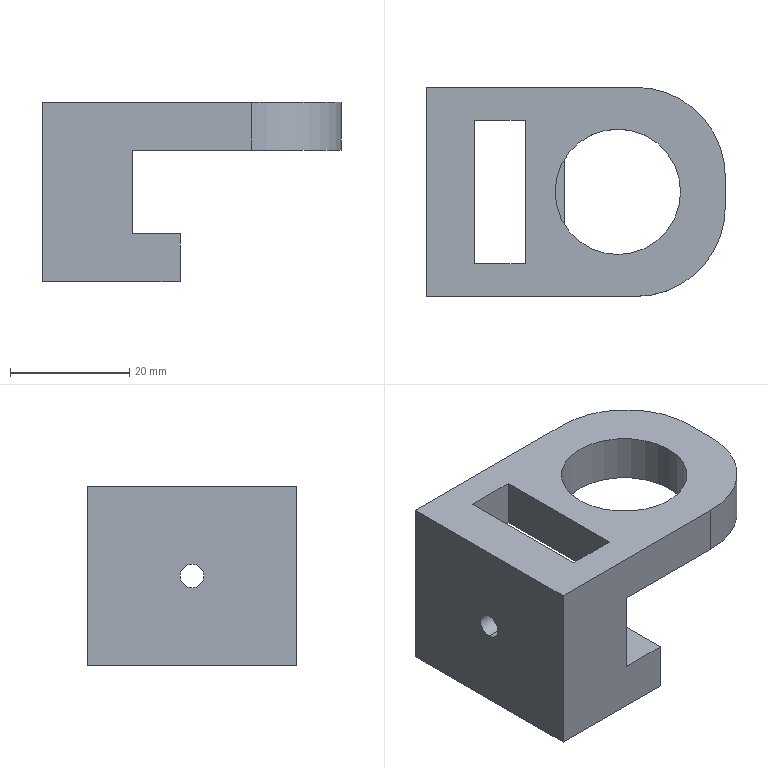Part | STEP file | X77-04004 | 1 solid | 22 faces | box 50 x 35 x 30 mm | volume 18530 mm3 | plane 16 | cylinder 6 | commonest cylinder face diameters 4 x2 21 x2 30 x2
STEP:
#1=CARTESIAN_POINT('',(0.,17.5,17.));
#2=VERTEX_POINT('',#1);
#3=CARTESIAN_POINT('',(0.,17.5,13.));
#4=VERTEX_POINT('',#3);
#5=CARTESIAN_POINT('',(0.,17.5,15.));
#6=DIRECTION('',(1.,0.,0.));
#7=DIRECTION('',(0.,0.,-1.));
#8=AXIS2_PLACEMENT_3D('',#5,#6,#7);
#9=CIRCLE('',#8,2.);
#10=EDGE_CURVE('',#2,#4,#9,.T.);
#11=ORIENTED_EDGE('',*,*,#10,.F.);
#12=CARTESIAN_POINT('',(8.,17.5,17.));
#13=VERTEX_POINT('',#12);
#14=CARTESIAN_POINT('',(8.,17.5,17.));
#15=DIRECTION('',(1.,0.,0.));
#16=VECTOR('',#15,1000.);
#17=LINE('',#14,#16);
#18=EDGE_CURVE('',#2,#13,#17,.T.);
#19=ORIENTED_EDGE('',*,*,#18,.T.);
#20=CARTESIAN_POINT('',(8.,17.5,13.));
#21=VERTEX_POINT('',#20);
#22=CARTESIAN_POINT('',(8.,17.5,15.));
#23=DIRECTION('',(1.,0.,0.));
#24=DIRECTION('',(0.,0.,-1.));
#25=AXIS2_PLACEMENT_3D('',#22,#23,#24);
#26=CIRCLE('',#25,2.);
#27=EDGE_CURVE('',#13,#21,#26,.T.);
#28=ORIENTED_EDGE('',*,*,#27,.T.);
#29=CARTESIAN_POINT('',(8.,17.5,13.));
#30=DIRECTION('',(1.,0.,0.));
#31=VECTOR('',#30,1000.);
#32=LINE('',#29,#31);
#33=EDGE_CURVE('',#4,#21,#32,.T.);
#34=ORIENTED_EDGE('',*,*,#33,.F.);
#35=EDGE_LOOP('',(#11,#19,#28,#34));
#36=FACE_OUTER_BOUND('',#35,.T.);
#37=CARTESIAN_POINT('',(8.,17.5,15.));
#38=DIRECTION('',(1.,0.,0.));
#39=DIRECTION('',(0.,0.,-1.));
#40=AXIS2_PLACEMENT_3D('',#37,#38,#39);
#41=CYLINDRICAL_SURFACE('',#40,2.);
#42=ADVANCED_FACE('',(#36),#41,.F.);
#43=CARTESIAN_POINT('',(42.5,17.5,22.));
#44=VERTEX_POINT('',#43);
#45=CARTESIAN_POINT('',(21.5,17.5,22.));
#46=VERTEX_POINT('',#45);
#47=CARTESIAN_POINT('',(32.,17.5,22.));
#48=DIRECTION('',(0.,0.,-1.));
#49=DIRECTION('',(1.,0.,0.));
#50=AXIS2_PLACEMENT_3D('',#47,#48,#49);
#51=CIRCLE('',#50,10.5);
#52=EDGE_CURVE('',#44,#46,#51,.T.);
#53=ORIENTED_EDGE('',*,*,#52,.T.);
#54=CARTESIAN_POINT('',(21.5,17.5,30.));
#55=VERTEX_POINT('',#54);
#56=CARTESIAN_POINT('',(21.5,17.5,-0.001));
#57=DIRECTION('',(0.,0.,1.));
#58=VECTOR('',#57,1000.);
#59=LINE('',#56,#58);
#60=EDGE_CURVE('',#46,#55,#59,.T.);
#61=ORIENTED_EDGE('',*,*,#60,.T.);
#62=CARTESIAN_POINT('',(42.5,17.5,30.));
#63=VERTEX_POINT('',#62);
#64=CARTESIAN_POINT('',(32.,17.5,30.));
#65=DIRECTION('',(0.,0.,1.));
#66=DIRECTION('',(1.,0.,0.));
#67=AXIS2_PLACEMENT_3D('',#64,#65,#66);
#68=CIRCLE('',#67,10.5);
#69=EDGE_CURVE('',#55,#63,#68,.T.);
#70=ORIENTED_EDGE('',*,*,#69,.T.);
#71=CARTESIAN_POINT('',(42.5,17.5,-0.001));
#72=DIRECTION('',(0.,0.,1.));
#73=VECTOR('',#72,1000.);
#74=LINE('',#71,#73);
#75=EDGE_CURVE('',#44,#63,#74,.T.);
#76=ORIENTED_EDGE('',*,*,#75,.F.);
#77=EDGE_LOOP('',(#53,#61,#70,#76));
#78=FACE_OUTER_BOUND('',#77,.T.);
#79=CARTESIAN_POINT('',(32.,17.5,-0.001));
#80=DIRECTION('',(0.,0.,1.));
#81=DIRECTION('',(1.,0.,0.));
#82=AXIS2_PLACEMENT_3D('',#79,#80,#81);
#83=CYLINDRICAL_SURFACE('',#82,10.5);
#84=ADVANCED_FACE('',(#78),#83,.F.);
#85=CARTESIAN_POINT('',(16.5,5.5,22.));
#86=VERTEX_POINT('',#85);
#87=CARTESIAN_POINT('',(16.5,29.5,22.));
#88=VERTEX_POINT('',#87);
#89=CARTESIAN_POINT('',(16.5,29.5,22.));
#90=DIRECTION('',(0.,1.,0.));
#91=VECTOR('',#90,1000.);
#92=LINE('',#89,#91);
#93=EDGE_CURVE('',#86,#88,#92,.T.);
#94=ORIENTED_EDGE('',*,*,#93,.F.);
#95=CARTESIAN_POINT('',(16.5,5.5,30.));
#96=VERTEX_POINT('',#95);
#97=CARTESIAN_POINT('',(16.5,5.5,30.));
#98=DIRECTION('',(0.,0.,-1.));
#99=VECTOR('',#98,1000.);
#100=LINE('',#97,#99);
#101=EDGE_CURVE('',#96,#86,#100,.T.);
#102=ORIENTED_EDGE('',*,*,#101,.F.);
#103=CARTESIAN_POINT('',(16.5,29.5,30.));
#104=VERTEX_POINT('',#103);
#105=CARTESIAN_POINT('',(16.5,29.5,30.));
#106=DIRECTION('',(0.,1.,0.));
#107=VECTOR('',#106,1000.);
#108=LINE('',#105,#107);
#109=EDGE_CURVE('',#96,#104,#108,.T.);
#110=ORIENTED_EDGE('',*,*,#109,.T.);
#111=CARTESIAN_POINT('',(16.5,29.5,30.));
#112=DIRECTION('',(0.,0.,-1.));
#113=VECTOR('',#112,1000.);
#114=LINE('',#111,#113);
#115=EDGE_CURVE('',#104,#88,#114,.T.);
#116=ORIENTED_EDGE('',*,*,#115,.T.);
#117=EDGE_LOOP('',(#94,#102,#110,#116));
#118=FACE_OUTER_BOUND('',#117,.T.);
#119=CARTESIAN_POINT('',(16.5,29.5,30.));
#120=DIRECTION('',(-1.,0.,0.));
#121=DIRECTION('',(0.,-1.,0.));
#122=AXIS2_PLACEMENT_3D('',#119,#120,#121);
#123=PLANE('',#122);
#124=ADVANCED_FACE('',(#118),#123,.T.);
#125=CARTESIAN_POINT('',(32.,17.5,30.));
#126=DIRECTION('',(0.,0.,1.));
#127=DIRECTION('',(1.,0.,0.));
#128=AXIS2_PLACEMENT_3D('',#125,#126,#127);
#129=CIRCLE('',#128,10.5);
#130=EDGE_CURVE('',#63,#55,#129,.T.);
#131=ORIENTED_EDGE('',*,*,#130,.F.);
#132=ORIENTED_EDGE('',*,*,#69,.F.);
#133=EDGE_LOOP('',(#131,#132));
#134=FACE_BOUND('',#133,.T.);
#135=CARTESIAN_POINT('',(0.,0.,30.));
#136=VERTEX_POINT('',#135);
#137=CARTESIAN_POINT('',(35.,0.,30.));
#138=VERTEX_POINT('',#137);
#139=CARTESIAN_POINT('',(0.,0.,30.));
#140=DIRECTION('',(1.,0.,0.));
#141=VECTOR('',#140,1000.);
#142=LINE('',#139,#141);
#143=EDGE_CURVE('',#136,#138,#142,.T.);
#144=ORIENTED_EDGE('',*,*,#143,.T.);
#145=CARTESIAN_POINT('',(50.,15.,30.));
#146=VERTEX_POINT('',#145);
#147=CARTESIAN_POINT('',(35.,15.,30.));
#148=DIRECTION('',(0.,0.,1.));
#149=DIRECTION('',(-1.,0.,0.));
#150=AXIS2_PLACEMENT_3D('',#147,#148,#149);
#151=CIRCLE('',#150,15.);
#152=EDGE_CURVE('',#138,#146,#151,.T.);
#153=ORIENTED_EDGE('',*,*,#152,.T.);
#154=CARTESIAN_POINT('',(50.,20.,30.));
#155=VERTEX_POINT('',#154);
#156=CARTESIAN_POINT('',(50.,0.,30.));
#157=DIRECTION('',(0.,1.,0.));
#158=VECTOR('',#157,1000.);
#159=LINE('',#156,#158);
#160=EDGE_CURVE('',#146,#155,#159,.T.);
#161=ORIENTED_EDGE('',*,*,#160,.T.);
#162=CARTESIAN_POINT('',(35.,35.,30.));
#163=VERTEX_POINT('',#162);
#164=CARTESIAN_POINT('',(35.,20.,30.));
#165=DIRECTION('',(0.,0.,1.));
#166=DIRECTION('',(-1.,0.,0.));
#167=AXIS2_PLACEMENT_3D('',#164,#165,#166);
#168=CIRCLE('',#167,15.);
#169=EDGE_CURVE('',#155,#163,#168,.T.);
#170=ORIENTED_EDGE('',*,*,#169,.T.);
#171=CARTESIAN_POINT('',(0.,35.,30.));
#172=VERTEX_POINT('',#171);
#173=CARTESIAN_POINT('',(0.,35.,30.));
#174=DIRECTION('',(-1.,0.,0.));
#175=VECTOR('',#174,1000.);
#176=LINE('',#173,#175);
#177=EDGE_CURVE('',#163,#172,#176,.T.);
#178=ORIENTED_EDGE('',*,*,#177,.T.);
#179=CARTESIAN_POINT('',(0.,0.,30.));
#180=DIRECTION('',(0.,-1.,0.));
#181=VECTOR('',#180,1000.);
#182=LINE('',#179,#181);
#183=EDGE_CURVE('',#172,#136,#182,.T.);
#184=ORIENTED_EDGE('',*,*,#183,.T.);
#185=EDGE_LOOP('',(#144,#153,#161,#170,#178,#184));
#186=FACE_OUTER_BOUND('',#185,.T.);
#187=CARTESIAN_POINT('',(8.,29.5,30.));
#188=VERTEX_POINT('',#187);
#189=CARTESIAN_POINT('',(8.,5.5,30.));
#190=VERTEX_POINT('',#189);
#191=CARTESIAN_POINT('',(8.,29.5,30.));
#192=DIRECTION('',(0.,-1.,0.));
#193=VECTOR('',#192,1000.);
#194=LINE('',#191,#193);
#195=EDGE_CURVE('',#188,#190,#194,.T.);
#196=ORIENTED_EDGE('',*,*,#195,.F.);
#197=CARTESIAN_POINT('',(8.,29.5,30.));
#198=DIRECTION('',(-1.,0.,0.));
#199=VECTOR('',#198,1000.);
#200=LINE('',#197,#199);
#201=EDGE_CURVE('',#104,#188,#200,.T.);
#202=ORIENTED_EDGE('',*,*,#201,.F.);
#203=ORIENTED_EDGE('',*,*,#109,.F.);
#204=CARTESIAN_POINT('',(8.,5.5,30.));
#205=DIRECTION('',(1.,0.,0.));
#206=VECTOR('',#205,1000.);
#207=LINE('',#204,#206);
#208=EDGE_CURVE('',#190,#96,#207,.T.);
#209=ORIENTED_EDGE('',*,*,#208,.F.);
#210=EDGE_LOOP('',(#196,#202,#203,#209));
#211=FACE_BOUND('',#210,.T.);
#212=CARTESIAN_POINT('',(0.,35.,30.));
#213=DIRECTION('',(0.,0.,-1.));
#214=DIRECTION('',(-1.,0.,0.));
#215=AXIS2_PLACEMENT_3D('',#212,#213,#214);
#216=PLANE('',#215);
#217=ADVANCED_FACE('',(#134,#186,#211),#216,.F.);
#218=CARTESIAN_POINT('',(23.,35.,0.));
#219=VERTEX_POINT('',#218);
#220=CARTESIAN_POINT('',(23.,0.,0.));
#221=VERTEX_POINT('',#220);
#222=CARTESIAN_POINT('',(23.,44.,0.));
#223=DIRECTION('',(0.,-1.,0.));
#224=VECTOR('',#223,1000.);
#225=LINE('',#222,#224);
#226=EDGE_CURVE('',#219,#221,#225,.T.);
#227=ORIENTED_EDGE('',*,*,#226,.T.);
#228=CARTESIAN_POINT('',(0.,0.,0.));
#229=VERTEX_POINT('',#228);
#230=CARTESIAN_POINT('',(0.,0.,0.));
#231=DIRECTION('',(1.,0.,0.));
#232=VECTOR('',#231,1000.);
#233=LINE('',#230,#232);
#234=EDGE_CURVE('',#229,#221,#233,.T.);
#235=ORIENTED_EDGE('',*,*,#234,.F.);
#236=CARTESIAN_POINT('',(0.,35.,0.));
#237=VERTEX_POINT('',#236);
#238=CARTESIAN_POINT('',(0.,0.,0.));
#239=DIRECTION('',(0.,-1.,0.));
#240=VECTOR('',#239,1000.);
#241=LINE('',#238,#240);
#242=EDGE_CURVE('',#237,#229,#241,.T.);
#243=ORIENTED_EDGE('',*,*,#242,.F.);
#244=CARTESIAN_POINT('',(0.,35.,0.));
#245=DIRECTION('',(-1.,0.,0.));
#246=VECTOR('',#245,1000.);
#247=LINE('',#244,#246);
#248=EDGE_CURVE('',#219,#237,#247,.T.);
#249=ORIENTED_EDGE('',*,*,#248,.F.);
#250=EDGE_LOOP('',(#227,#235,#243,#249));
#251=FACE_OUTER_BOUND('',#250,.T.);
#252=CARTESIAN_POINT('',(16.5,29.5,0.));
#253=VERTEX_POINT('',#252);
#254=CARTESIAN_POINT('',(8.,29.5,0.));
#255=VERTEX_POINT('',#254);
#256=CARTESIAN_POINT('',(8.,29.5,0.));
#257=DIRECTION('',(-1.,0.,0.));
#258=VECTOR('',#257,1000.);
#259=LINE('',#256,#258);
#260=EDGE_CURVE('',#253,#255,#259,.T.);
#261=ORIENTED_EDGE('',*,*,#260,.T.);
#262=CARTESIAN_POINT('',(8.,5.5,0.));
#263=VERTEX_POINT('',#262);
#264=CARTESIAN_POINT('',(8.,29.5,0.));
#265=DIRECTION('',(0.,-1.,0.));
#266=VECTOR('',#265,1000.);
#267=LINE('',#264,#266);
#268=EDGE_CURVE('',#255,#263,#267,.T.);
#269=ORIENTED_EDGE('',*,*,#268,.T.);
#270=CARTESIAN_POINT('',(16.5,5.5,0.));
#271=VERTEX_POINT('',#270);
#272=CARTESIAN_POINT('',(8.,5.5,0.));
#273=DIRECTION('',(1.,0.,0.));
#274=VECTOR('',#273,1000.);
#275=LINE('',#272,#274);
#276=EDGE_CURVE('',#263,#271,#275,.T.);
#277=ORIENTED_EDGE('',*,*,#276,.T.);
#278=CARTESIAN_POINT('',(16.5,29.5,0.));
#279=DIRECTION('',(0.,1.,0.));
#280=VECTOR('',#279,1000.);
#281=LINE('',#278,#280);
#282=EDGE_CURVE('',#271,#253,#281,.T.);
#283=ORIENTED_EDGE('',*,*,#282,.T.);
#284=EDGE_LOOP('',(#261,#269,#277,#283));
#285=FACE_BOUND('',#284,.T.);
#286=CARTESIAN_POINT('',(0.,35.,0.));
#287=DIRECTION('',(0.,0.,-1.));
#288=DIRECTION('',(-1.,0.,0.));
#289=AXIS2_PLACEMENT_3D('',#286,#287,#288);
#290=PLANE('',#289);
#291=ADVANCED_FACE('',(#251,#285),#290,.T.);
#292=CARTESIAN_POINT('',(0.,17.5,15.));
#293=DIRECTION('',(1.,0.,0.));
#294=DIRECTION('',(0.,0.,-1.));
#295=AXIS2_PLACEMENT_3D('',#292,#293,#294);
#296=CIRCLE('',#295,2.);
#297=EDGE_CURVE('',#4,#2,#296,.T.);
#298=ORIENTED_EDGE('',*,*,#297,.T.);
#299=ORIENTED_EDGE('',*,*,#10,.T.);
#300=EDGE_LOOP('',(#298,#299));
#301=FACE_BOUND('',#300,.T.);
#302=ORIENTED_EDGE('',*,*,#242,.T.);
#303=CARTESIAN_POINT('',(0.,0.,30.));
#304=DIRECTION('',(0.,0.,-1.));
#305=VECTOR('',#304,1000.);
#306=LINE('',#303,#305);
#307=EDGE_CURVE('',#136,#229,#306,.T.);
#308=ORIENTED_EDGE('',*,*,#307,.F.);
#309=ORIENTED_EDGE('',*,*,#183,.F.);
#310=CARTESIAN_POINT('',(0.,35.,30.));
#311=DIRECTION('',(0.,0.,-1.));
#312=VECTOR('',#311,1000.);
#313=LINE('',#310,#312);
#314=EDGE_CURVE('',#172,#237,#313,.T.);
#315=ORIENTED_EDGE('',*,*,#314,.T.);
#316=EDGE_LOOP('',(#302,#308,#309,#315));
#317=FACE_OUTER_BOUND('',#316,.T.);
#318=CARTESIAN_POINT('',(0.,0.,30.));
#319=DIRECTION('',(1.,0.,0.));
#320=DIRECTION('',(0.,0.,-1.));
#321=AXIS2_PLACEMENT_3D('',#318,#319,#320);
#322=PLANE('',#321);
#323=ADVANCED_FACE('',(#301,#317),#322,.F.);
#324=CARTESIAN_POINT('',(35.,0.,22.));
#325=VERTEX_POINT('',#324);
#326=CARTESIAN_POINT('',(15.,0.,22.));
#327=VERTEX_POINT('',#326);
#328=CARTESIAN_POINT('',(50.,0.,22.));
#329=DIRECTION('',(-1.,0.,0.));
#330=VECTOR('',#329,1000.);
#331=LINE('',#328,#330);
#332=EDGE_CURVE('',#325,#327,#331,.T.);
#333=ORIENTED_EDGE('',*,*,#332,.F.);
#334=CARTESIAN_POINT('',(35.,0.,30.));
#335=DIRECTION('',(0.,0.,1.));
#336=VECTOR('',#335,1000.);
#337=LINE('',#334,#336);
#338=EDGE_CURVE('',#325,#138,#337,.T.);
#339=ORIENTED_EDGE('',*,*,#338,.T.);
#340=ORIENTED_EDGE('',*,*,#143,.F.);
#341=ORIENTED_EDGE('',*,*,#307,.T.);
#342=ORIENTED_EDGE('',*,*,#234,.T.);
#343=CARTESIAN_POINT('',(23.,0.,8.));
#344=VERTEX_POINT('',#343);
#345=CARTESIAN_POINT('',(23.,0.,8.));
#346=DIRECTION('',(0.,0.,-1.));
#347=VECTOR('',#346,1000.);
#348=LINE('',#345,#347);
#349=EDGE_CURVE('',#344,#221,#348,.T.);
#350=ORIENTED_EDGE('',*,*,#349,.F.);
#351=CARTESIAN_POINT('',(15.,0.,8.));
#352=VERTEX_POINT('',#351);
#353=CARTESIAN_POINT('',(23.,0.,8.));
#354=DIRECTION('',(1.,0.,0.));
#355=VECTOR('',#354,1000.);
#356=LINE('',#353,#355);
#357=EDGE_CURVE('',#352,#344,#356,.T.);
#358=ORIENTED_EDGE('',*,*,#357,.F.);
#359=CARTESIAN_POINT('',(15.,0.,8.));
#360=DIRECTION('',(0.,0.,-1.));
#361=VECTOR('',#360,1000.);
#362=LINE('',#359,#361);
#363=EDGE_CURVE('',#327,#352,#362,.T.);
#364=ORIENTED_EDGE('',*,*,#363,.F.);
#365=EDGE_LOOP('',(#333,#339,#340,#341,#342,#350,#358,#364));
#366=FACE_OUTER_BOUND('',#365,.T.);
#367=CARTESIAN_POINT('',(0.,0.,30.));
#368=DIRECTION('',(0.,1.,0.));
#369=DIRECTION('',(0.,0.,1.));
#370=AXIS2_PLACEMENT_3D('',#367,#368,#369);
#371=PLANE('',#370);
#372=ADVANCED_FACE('',(#366),#371,.F.);
#373=ORIENTED_EDGE('',*,*,#160,.F.);
#374=CARTESIAN_POINT('',(50.,15.,22.));
#375=VERTEX_POINT('',#374);
#376=CARTESIAN_POINT('',(50.,15.,30.));
#377=DIRECTION('',(0.,0.,-1.));
#378=VECTOR('',#377,1000.);
#379=LINE('',#376,#378);
#380=EDGE_CURVE('',#146,#375,#379,.T.);
#381=ORIENTED_EDGE('',*,*,#380,.T.);
#382=CARTESIAN_POINT('',(50.,20.,22.));
#383=VERTEX_POINT('',#382);
#384=CARTESIAN_POINT('',(50.,44.,22.));
#385=DIRECTION('',(0.,-1.,0.));
#386=VECTOR('',#385,1000.);
#387=LINE('',#384,#386);
#388=EDGE_CURVE('',#383,#375,#387,.T.);
#389=ORIENTED_EDGE('',*,*,#388,.F.);
#390=CARTESIAN_POINT('',(50.,20.,30.));
#391=DIRECTION('',(0.,0.,1.));
#392=VECTOR('',#391,1000.);
#393=LINE('',#390,#392);
#394=EDGE_CURVE('',#383,#155,#393,.T.);
#395=ORIENTED_EDGE('',*,*,#394,.T.);
#396=EDGE_LOOP('',(#373,#381,#389,#395));
#397=FACE_OUTER_BOUND('',#396,.T.);
#398=CARTESIAN_POINT('',(50.,0.,30.));
#399=DIRECTION('',(-1.,0.,0.));
#400=DIRECTION('',(0.,0.,1.));
#401=AXIS2_PLACEMENT_3D('',#398,#399,#400);
#402=PLANE('',#401);
#403=ADVANCED_FACE('',(#397),#402,.F.);
#404=ORIENTED_EDGE('',*,*,#177,.F.);
#405=CARTESIAN_POINT('',(35.,35.,22.));
#406=VERTEX_POINT('',#405);
#407=CARTESIAN_POINT('',(35.,35.,30.));
#408=DIRECTION('',(0.,0.,-1.));
#409=VECTOR('',#408,1000.);
#410=LINE('',#407,#409);
#411=EDGE_CURVE('',#163,#406,#410,.T.);
#412=ORIENTED_EDGE('',*,*,#411,.T.);
#413=CARTESIAN_POINT('',(15.,35.,22.));
#414=VERTEX_POINT('',#413);
#415=CARTESIAN_POINT('',(0.,35.,22.));
#416=DIRECTION('',(-1.,0.,0.));
#417=VECTOR('',#416,1000.);
#418=LINE('',#415,#417);
#419=EDGE_CURVE('',#406,#414,#418,.T.);
#420=ORIENTED_EDGE('',*,*,#419,.T.);
#421=CARTESIAN_POINT('',(15.,35.,8.));
#422=VERTEX_POINT('',#421);
#423=CARTESIAN_POINT('',(15.,35.,30.));
#424=DIRECTION('',(0.,0.,-1.));
#425=VECTOR('',#424,1000.);
#426=LINE('',#423,#425);
#427=EDGE_CURVE('',#414,#422,#426,.T.);
#428=ORIENTED_EDGE('',*,*,#427,.T.);
#429=CARTESIAN_POINT('',(23.,35.,8.));
#430=VERTEX_POINT('',#429);
#431=CARTESIAN_POINT('',(0.,35.,8.));
#432=DIRECTION('',(1.,0.,0.));
#433=VECTOR('',#432,1000.);
#434=LINE('',#431,#433);
#435=EDGE_CURVE('',#422,#430,#434,.T.);
#436=ORIENTED_EDGE('',*,*,#435,.T.);
#437=CARTESIAN_POINT('',(23.,35.,30.));
#438=DIRECTION('',(0.,0.,-1.));
#439=VECTOR('',#438,1000.);
#440=LINE('',#437,#439);
#441=EDGE_CURVE('',#430,#219,#440,.T.);
#442=ORIENTED_EDGE('',*,*,#441,.T.);
#443=ORIENTED_EDGE('',*,*,#248,.T.);
#444=ORIENTED_EDGE('',*,*,#314,.F.);
#445=EDGE_LOOP('',(#404,#412,#420,#428,#436,#442,#443,#444));
#446=FACE_OUTER_BOUND('',#445,.T.);
#447=CARTESIAN_POINT('',(0.,35.,30.));
#448=DIRECTION('',(0.,-1.,0.));
#449=DIRECTION('',(0.,0.,-1.));
#450=AXIS2_PLACEMENT_3D('',#447,#448,#449);
#451=PLANE('',#450);
#452=ADVANCED_FACE('',(#446),#451,.F.);
#453=CARTESIAN_POINT('',(8.,17.5,15.));
#454=DIRECTION('',(1.,0.,0.));
#455=DIRECTION('',(0.,0.,-1.));
#456=AXIS2_PLACEMENT_3D('',#453,#454,#455);
#457=CIRCLE('',#456,2.);
#458=EDGE_CURVE('',#21,#13,#457,.T.);
#459=ORIENTED_EDGE('',*,*,#458,.F.);
#460=ORIENTED_EDGE('',*,*,#27,.F.);
#461=EDGE_LOOP('',(#459,#460));
#462=FACE_BOUND('',#461,.T.);
#463=ORIENTED_EDGE('',*,*,#268,.F.);
#464=CARTESIAN_POINT('',(8.,29.5,30.));
#465=DIRECTION('',(0.,0.,-1.));
#466=VECTOR('',#465,1000.);
#467=LINE('',#464,#466);
#468=EDGE_CURVE('',#188,#255,#467,.T.);
#469=ORIENTED_EDGE('',*,*,#468,.F.);
#470=ORIENTED_EDGE('',*,*,#195,.T.);
#471=CARTESIAN_POINT('',(8.,5.5,30.));
#472=DIRECTION('',(0.,0.,-1.));
#473=VECTOR('',#472,1000.);
#474=LINE('',#471,#473);
#475=EDGE_CURVE('',#190,#263,#474,.T.);
#476=ORIENTED_EDGE('',*,*,#475,.T.);
#477=EDGE_LOOP('',(#463,#469,#470,#476));
#478=FACE_OUTER_BOUND('',#477,.T.);
#479=CARTESIAN_POINT('',(8.,29.5,30.));
#480=DIRECTION('',(1.,0.,0.));
#481=DIRECTION('',(0.,1.,0.));
#482=AXIS2_PLACEMENT_3D('',#479,#480,#481);
#483=PLANE('',#482);
#484=ADVANCED_FACE('',(#462,#478),#483,.T.);
#485=CARTESIAN_POINT('',(15.,5.5,22.));
#486=VERTEX_POINT('',#485);
#487=CARTESIAN_POINT('',(8.,5.5,22.));
#488=DIRECTION('',(1.,0.,0.));
#489=VECTOR('',#488,1000.);
#490=LINE('',#487,#489);
#491=EDGE_CURVE('',#486,#86,#490,.T.);
#492=ORIENTED_EDGE('',*,*,#491,.F.);
#493=CARTESIAN_POINT('',(15.,5.5,8.));
#494=VERTEX_POINT('',#493);
#495=CARTESIAN_POINT('',(15.,5.5,30.));
#496=DIRECTION('',(0.,0.,1.));
#497=VECTOR('',#496,1000.);
#498=LINE('',#495,#497);
#499=EDGE_CURVE('',#494,#486,#498,.T.);
#500=ORIENTED_EDGE('',*,*,#499,.F.);
#501=CARTESIAN_POINT('',(16.5,5.5,8.));
#502=VERTEX_POINT('',#501);
#503=CARTESIAN_POINT('',(8.,5.5,8.));
#504=DIRECTION('',(-1.,0.,0.));
#505=VECTOR('',#504,1000.);
#506=LINE('',#503,#505);
#507=EDGE_CURVE('',#502,#494,#506,.T.);
#508=ORIENTED_EDGE('',*,*,#507,.F.);
#509=CARTESIAN_POINT('',(16.5,5.5,30.));
#510=DIRECTION('',(0.,0.,-1.));
#511=VECTOR('',#510,1000.);
#512=LINE('',#509,#511);
#513=EDGE_CURVE('',#502,#271,#512,.T.);
#514=ORIENTED_EDGE('',*,*,#513,.T.);
#515=ORIENTED_EDGE('',*,*,#276,.F.);
#516=ORIENTED_EDGE('',*,*,#475,.F.);
#517=ORIENTED_EDGE('',*,*,#208,.T.);
#518=ORIENTED_EDGE('',*,*,#101,.T.);
#519=EDGE_LOOP('',(#492,#500,#508,#514,#515,#516,#517,#518));
#520=FACE_OUTER_BOUND('',#519,.T.);
#521=CARTESIAN_POINT('',(8.,5.5,30.));
#522=DIRECTION('',(0.,1.,0.));
#523=DIRECTION('',(0.,0.,1.));
#524=AXIS2_PLACEMENT_3D('',#521,#522,#523);
#525=PLANE('',#524);
#526=ADVANCED_FACE('',(#520),#525,.T.);
#527=CARTESIAN_POINT('',(16.5,29.5,8.));
#528=VERTEX_POINT('',#527);
#529=CARTESIAN_POINT('',(16.5,29.5,8.));
#530=DIRECTION('',(0.,-1.,0.));
#531=VECTOR('',#530,1000.);
#532=LINE('',#529,#531);
#533=EDGE_CURVE('',#528,#502,#532,.T.);
#534=ORIENTED_EDGE('',*,*,#533,.F.);
#535=CARTESIAN_POINT('',(16.5,29.5,30.));
#536=DIRECTION('',(0.,0.,-1.));
#537=VECTOR('',#536,1000.);
#538=LINE('',#535,#537);
#539=EDGE_CURVE('',#528,#253,#538,.T.);
#540=ORIENTED_EDGE('',*,*,#539,.T.);
#541=ORIENTED_EDGE('',*,*,#282,.F.);
#542=ORIENTED_EDGE('',*,*,#513,.F.);
#543=EDGE_LOOP('',(#534,#540,#541,#542));
#544=FACE_OUTER_BOUND('',#543,.T.);
#545=CARTESIAN_POINT('',(16.5,29.5,30.));
#546=DIRECTION('',(-1.,0.,0.));
#547=DIRECTION('',(0.,-1.,0.));
#548=AXIS2_PLACEMENT_3D('',#545,#546,#547);
#549=PLANE('',#548);
#550=ADVANCED_FACE('',(#544),#549,.T.);
#551=CARTESIAN_POINT('',(15.,29.5,22.));
#552=VERTEX_POINT('',#551);
#553=CARTESIAN_POINT('',(8.,29.5,22.));
#554=DIRECTION('',(-1.,0.,0.));
#555=VECTOR('',#554,1000.);
#556=LINE('',#553,#555);
#557=EDGE_CURVE('',#88,#552,#556,.T.);
#558=ORIENTED_EDGE('',*,*,#557,.F.);
#559=ORIENTED_EDGE('',*,*,#115,.F.);
#560=ORIENTED_EDGE('',*,*,#201,.T.);
#561=ORIENTED_EDGE('',*,*,#468,.T.);
#562=ORIENTED_EDGE('',*,*,#260,.F.);
#563=ORIENTED_EDGE('',*,*,#539,.F.);
#564=CARTESIAN_POINT('',(15.,29.5,8.));
#565=VERTEX_POINT('',#564);
#566=CARTESIAN_POINT('',(8.,29.5,8.));
#567=DIRECTION('',(1.,0.,0.));
#568=VECTOR('',#567,1000.);
#569=LINE('',#566,#568);
#570=EDGE_CURVE('',#565,#528,#569,.T.);
#571=ORIENTED_EDGE('',*,*,#570,.F.);
#572=CARTESIAN_POINT('',(15.,29.5,30.));
#573=DIRECTION('',(0.,0.,-1.));
#574=VECTOR('',#573,1000.);
#575=LINE('',#572,#574);
#576=EDGE_CURVE('',#552,#565,#575,.T.);
#577=ORIENTED_EDGE('',*,*,#576,.F.);
#578=EDGE_LOOP('',(#558,#559,#560,#561,#562,#563,#571,#577));
#579=FACE_OUTER_BOUND('',#578,.T.);
#580=CARTESIAN_POINT('',(8.,29.5,30.));
#581=DIRECTION('',(0.,-1.,0.));
#582=DIRECTION('',(0.,0.,-1.));
#583=AXIS2_PLACEMENT_3D('',#580,#581,#582);
#584=PLANE('',#583);
#585=ADVANCED_FACE('',(#579),#584,.T.);
#586=CARTESIAN_POINT('',(23.,44.,8.));
#587=DIRECTION('',(0.,-1.,0.));
#588=VECTOR('',#587,1000.);
#589=LINE('',#586,#588);
#590=EDGE_CURVE('',#430,#344,#589,.T.);
#591=ORIENTED_EDGE('',*,*,#590,.T.);
#592=ORIENTED_EDGE('',*,*,#349,.T.);
#593=ORIENTED_EDGE('',*,*,#226,.F.);
#594=ORIENTED_EDGE('',*,*,#441,.F.);
#595=EDGE_LOOP('',(#591,#592,#593,#594));
#596=FACE_OUTER_BOUND('',#595,.T.);
#597=CARTESIAN_POINT('',(23.,44.,8.));
#598=DIRECTION('',(-1.,0.,0.));
#599=DIRECTION('',(0.,0.,1.));
#600=AXIS2_PLACEMENT_3D('',#597,#598,#599);
#601=PLANE('',#600);
#602=ADVANCED_FACE('',(#596),#601,.F.);
#603=CARTESIAN_POINT('',(15.,44.,22.));
#604=DIRECTION('',(0.,-1.,0.));
#605=VECTOR('',#604,1000.);
#606=LINE('',#603,#605);
#607=EDGE_CURVE('',#414,#552,#606,.T.);
#608=ORIENTED_EDGE('',*,*,#607,.T.);
#609=ORIENTED_EDGE('',*,*,#576,.T.);
#610=CARTESIAN_POINT('',(15.,44.,8.));
#611=DIRECTION('',(0.,-1.,0.));
#612=VECTOR('',#611,1000.);
#613=LINE('',#610,#612);
#614=EDGE_CURVE('',#422,#565,#613,.T.);
#615=ORIENTED_EDGE('',*,*,#614,.F.);
#616=ORIENTED_EDGE('',*,*,#427,.F.);
#617=EDGE_LOOP('',(#608,#609,#615,#616));
#618=FACE_OUTER_BOUND('',#617,.T.);
#619=CARTESIAN_POINT('',(15.,44.,8.));
#620=DIRECTION('',(-1.,0.,0.));
#621=DIRECTION('',(0.,0.,1.));
#622=AXIS2_PLACEMENT_3D('',#619,#620,#621);
#623=PLANE('',#622);
#624=ADVANCED_FACE('',(#618),#623,.F.);
#625=ORIENTED_EDGE('',*,*,#499,.T.);
#626=CARTESIAN_POINT('',(15.,44.,22.));
#627=DIRECTION('',(0.,-1.,0.));
#628=VECTOR('',#627,1000.);
#629=LINE('',#626,#628);
#630=EDGE_CURVE('',#486,#327,#629,.T.);
#631=ORIENTED_EDGE('',*,*,#630,.T.);
#632=ORIENTED_EDGE('',*,*,#363,.T.);
#633=CARTESIAN_POINT('',(15.,44.,8.));
#634=DIRECTION('',(0.,-1.,0.));
#635=VECTOR('',#634,1000.);
#636=LINE('',#633,#635);
#637=EDGE_CURVE('',#494,#352,#636,.T.);
#638=ORIENTED_EDGE('',*,*,#637,.F.);
#639=EDGE_LOOP('',(#625,#631,#632,#638));
#640=FACE_OUTER_BOUND('',#639,.T.);
#641=CARTESIAN_POINT('',(15.,44.,8.));
#642=DIRECTION('',(-1.,0.,0.));
#643=DIRECTION('',(0.,0.,1.));
#644=AXIS2_PLACEMENT_3D('',#641,#642,#643);
#645=PLANE('',#644);
#646=ADVANCED_FACE('',(#640),#645,.F.);
#647=ORIENTED_EDGE('',*,*,#52,.F.);
#648=CARTESIAN_POINT('',(32.,17.5,22.));
#649=DIRECTION('',(0.,0.,-1.));
#650=DIRECTION('',(1.,0.,0.));
#651=AXIS2_PLACEMENT_3D('',#648,#649,#650);
#652=CIRCLE('',#651,10.5);
#653=EDGE_CURVE('',#46,#44,#652,.T.);
#654=ORIENTED_EDGE('',*,*,#653,.F.);
#655=EDGE_LOOP('',(#647,#654));
#656=FACE_BOUND('',#655,.T.);
#657=ORIENTED_EDGE('',*,*,#388,.T.);
#658=CARTESIAN_POINT('',(35.,15.,22.));
#659=DIRECTION('',(0.,0.,-1.));
#660=DIRECTION('',(1.,0.,0.));
#661=AXIS2_PLACEMENT_3D('',#658,#659,#660);
#662=CIRCLE('',#661,15.);
#663=EDGE_CURVE('',#375,#325,#662,.T.);
#664=ORIENTED_EDGE('',*,*,#663,.T.);
#665=ORIENTED_EDGE('',*,*,#332,.T.);
#666=ORIENTED_EDGE('',*,*,#630,.F.);
#667=ORIENTED_EDGE('',*,*,#491,.T.);
#668=ORIENTED_EDGE('',*,*,#93,.T.);
#669=ORIENTED_EDGE('',*,*,#557,.T.);
#670=ORIENTED_EDGE('',*,*,#607,.F.);
#671=ORIENTED_EDGE('',*,*,#419,.F.);
#672=CARTESIAN_POINT('',(35.,20.,22.));
#673=DIRECTION('',(0.,0.,-1.));
#674=DIRECTION('',(1.,0.,0.));
#675=AXIS2_PLACEMENT_3D('',#672,#673,#674);
#676=CIRCLE('',#675,15.);
#677=EDGE_CURVE('',#406,#383,#676,.T.);
#678=ORIENTED_EDGE('',*,*,#677,.T.);
#679=EDGE_LOOP('',(#657,#664,#665,#666,#667,#668,#669,#670,#671,#678));
#680=FACE_OUTER_BOUND('',#679,.T.);
#681=CARTESIAN_POINT('',(50.,44.,22.));
#682=DIRECTION('',(0.,0.,1.));
#683=DIRECTION('',(1.,0.,0.));
#684=AXIS2_PLACEMENT_3D('',#681,#682,#683);
#685=PLANE('',#684);
#686=ADVANCED_FACE('',(#656,#680),#685,.F.);
#687=ORIENTED_EDGE('',*,*,#614,.T.);
#688=ORIENTED_EDGE('',*,*,#570,.T.);
#689=ORIENTED_EDGE('',*,*,#533,.T.);
#690=ORIENTED_EDGE('',*,*,#507,.T.);
#691=ORIENTED_EDGE('',*,*,#637,.T.);
#692=ORIENTED_EDGE('',*,*,#357,.T.);
#693=ORIENTED_EDGE('',*,*,#590,.F.);
#694=ORIENTED_EDGE('',*,*,#435,.F.);
#695=EDGE_LOOP('',(#687,#688,#689,#690,#691,#692,#693,#694));
#696=FACE_OUTER_BOUND('',#695,.T.);
#697=CARTESIAN_POINT('',(23.,44.,8.));
#698=DIRECTION('',(0.,0.,-1.));
#699=DIRECTION('',(-1.,0.,0.));
#700=AXIS2_PLACEMENT_3D('',#697,#698,#699);
#701=PLANE('',#700);
#702=ADVANCED_FACE('',(#696),#701,.F.);
#703=ORIENTED_EDGE('',*,*,#60,.F.);
#704=ORIENTED_EDGE('',*,*,#653,.T.);
#705=ORIENTED_EDGE('',*,*,#75,.T.);
#706=ORIENTED_EDGE('',*,*,#130,.T.);
#707=EDGE_LOOP('',(#703,#704,#705,#706));
#708=FACE_OUTER_BOUND('',#707,.T.);
#709=CARTESIAN_POINT('',(32.,17.5,-0.001));
#710=DIRECTION('',(0.,0.,1.));
#711=DIRECTION('',(1.,0.,0.));
#712=AXIS2_PLACEMENT_3D('',#709,#710,#711);
#713=CYLINDRICAL_SURFACE('',#712,10.5);
#714=ADVANCED_FACE('',(#708),#713,.F.);
#715=ORIENTED_EDGE('',*,*,#152,.F.);
#716=ORIENTED_EDGE('',*,*,#338,.F.);
#717=ORIENTED_EDGE('',*,*,#663,.F.);
#718=ORIENTED_EDGE('',*,*,#380,.F.);
#719=EDGE_LOOP('',(#715,#716,#717,#718));
#720=FACE_OUTER_BOUND('',#719,.T.);
#721=CARTESIAN_POINT('',(35.,15.,30.));
#722=DIRECTION('',(0.,0.,-1.));
#723=DIRECTION('',(-1.,0.,0.));
#724=AXIS2_PLACEMENT_3D('',#721,#722,#723);
#725=CYLINDRICAL_SURFACE('',#724,15.);
#726=ADVANCED_FACE('',(#720),#725,.T.);
#727=ORIENTED_EDGE('',*,*,#169,.F.);
#728=ORIENTED_EDGE('',*,*,#394,.F.);
#729=ORIENTED_EDGE('',*,*,#677,.F.);
#730=ORIENTED_EDGE('',*,*,#411,.F.);
#731=EDGE_LOOP('',(#727,#728,#729,#730));
#732=FACE_OUTER_BOUND('',#731,.T.);
#733=CARTESIAN_POINT('',(35.,20.,30.));
#734=DIRECTION('',(0.,0.,-1.));
#735=DIRECTION('',(-1.,0.,0.));
#736=AXIS2_PLACEMENT_3D('',#733,#734,#735);
#737=CYLINDRICAL_SURFACE('',#736,15.);
#738=ADVANCED_FACE('',(#732),#737,.T.);
#739=ORIENTED_EDGE('',*,*,#18,.F.);
#740=ORIENTED_EDGE('',*,*,#297,.F.);
#741=ORIENTED_EDGE('',*,*,#33,.T.);
#742=ORIENTED_EDGE('',*,*,#458,.T.);
#743=EDGE_LOOP('',(#739,#740,#741,#742));
#744=FACE_OUTER_BOUND('',#743,.T.);
#745=CARTESIAN_POINT('',(8.,17.5,15.));
#746=DIRECTION('',(1.,0.,0.));
#747=DIRECTION('',(0.,0.,-1.));
#748=AXIS2_PLACEMENT_3D('',#745,#746,#747);
#749=CYLINDRICAL_SURFACE('',#748,2.);
#750=ADVANCED_FACE('',(#744),#749,.F.);
#751=CLOSED_SHELL('',(#42,#84,#124,#217,#291,#323,#372,#403,#452,#484,#526,#550,#585,#602,#624,#646,#686,#702,#714,#726,#738,#750));
#752=MANIFOLD_SOLID_BREP('',#751);
#753=CARTESIAN_POINT('',(0.,0.,0.));
#754=DIRECTION('',(0.,0.,1.));
#755=DIRECTION('',(1.,0.,0.));
#756=AXIS2_PLACEMENT_3D('',#753,#754,#755);
#757=(LENGTH_UNIT()NAMED_UNIT(*)SI_UNIT(.MILLI.,.METRE.));
#758=UNCERTAINTY_MEASURE_WITH_UNIT(LENGTH_MEASURE(0.00001),#757,'','');
#759=(NAMED_UNIT(*)PLANE_ANGLE_UNIT()SI_UNIT($,.RADIAN.));
#760=(NAMED_UNIT(*)SI_UNIT($,.STERADIAN.)SOLID_ANGLE_UNIT());
#761=(GEOMETRIC_REPRESENTATION_CONTEXT(3)GLOBAL_UNCERTAINTY_ASSIGNED_CONTEXT((#758))GLOBAL_UNIT_ASSIGNED_CONTEXT((#757,#759,#760))REPRESENTATION_CONTEXT('',''));
#762=ADVANCED_BREP_SHAPE_REPRESENTATION('',(#752,#756),#761);